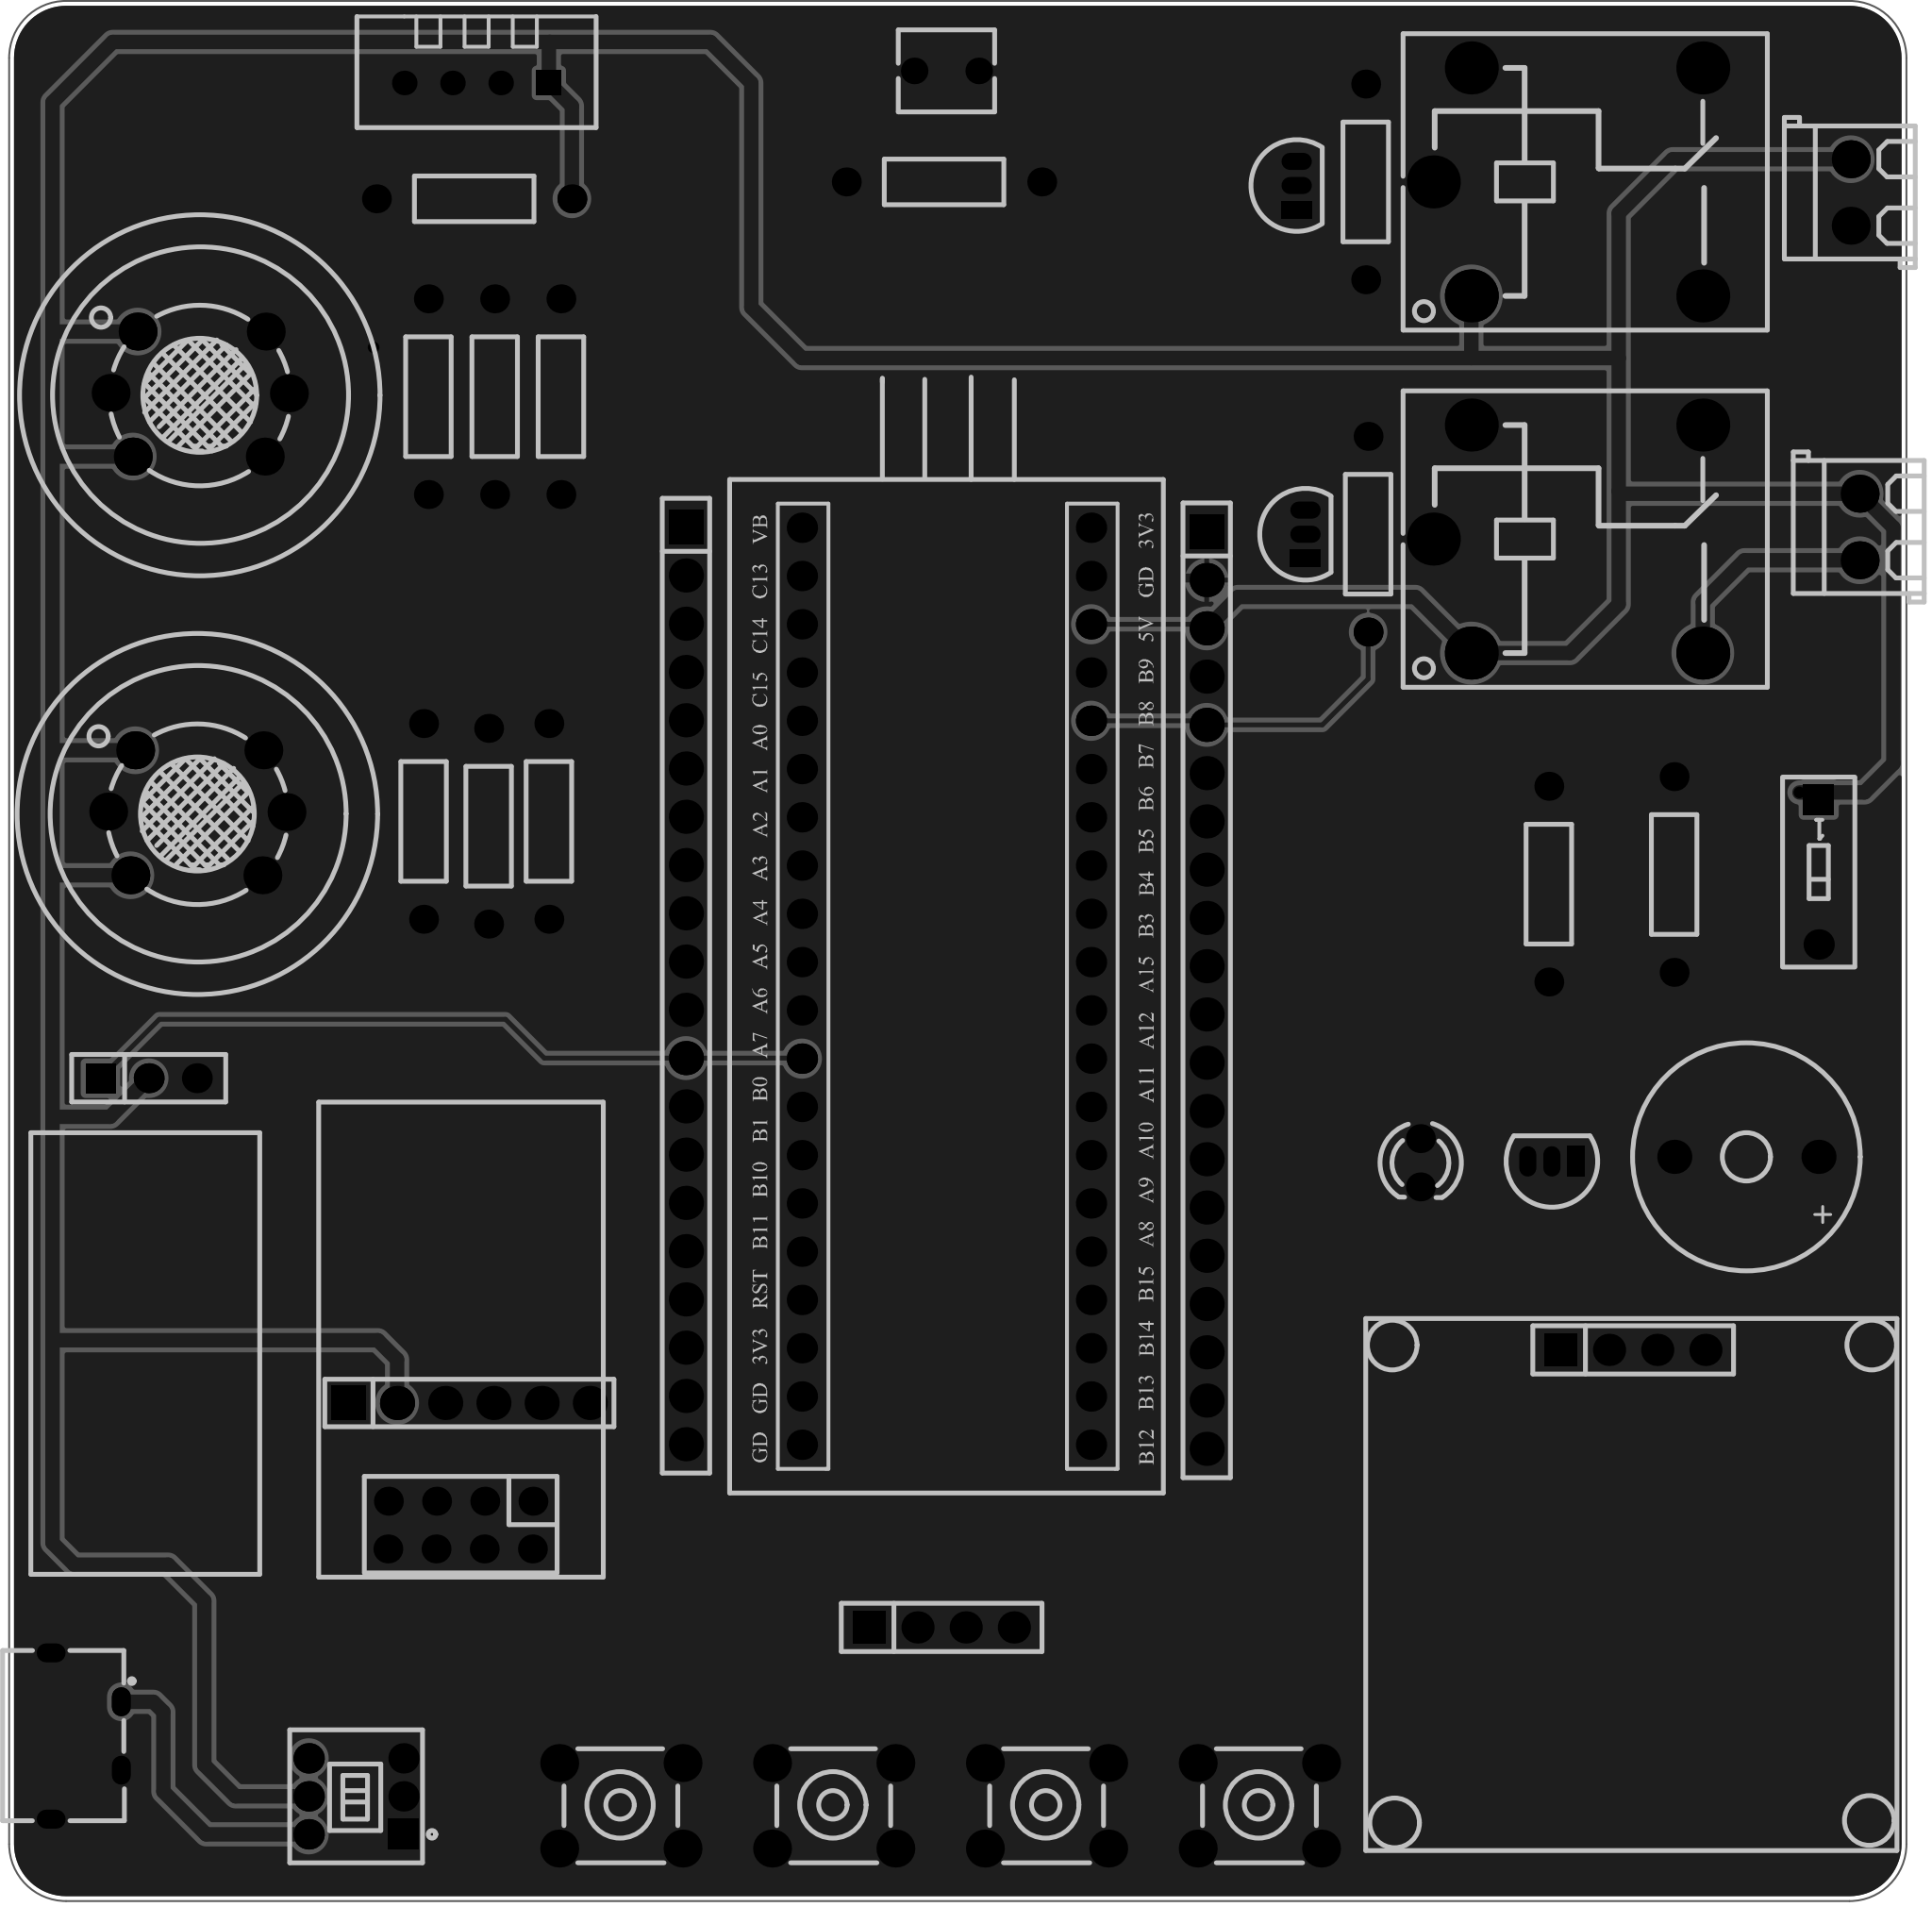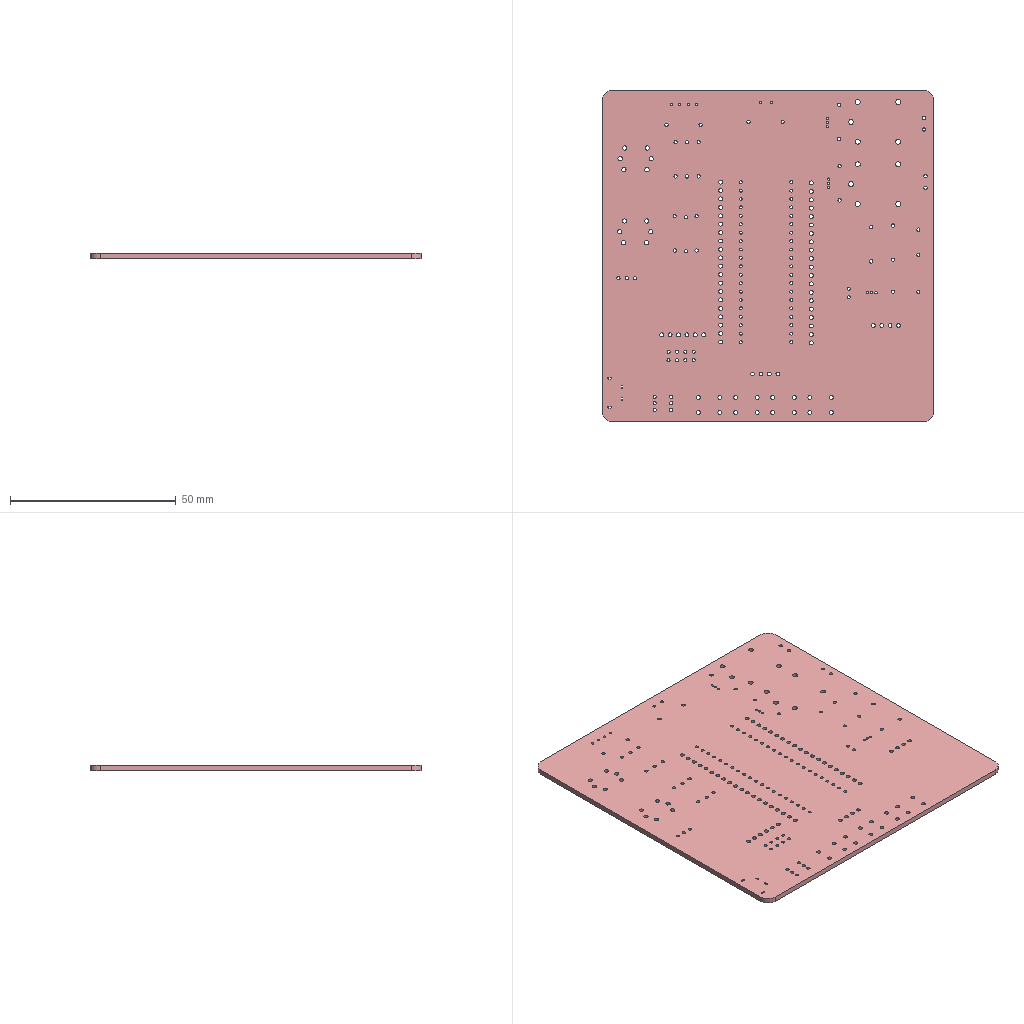Circuit board layout | Altium Designer | box 100 x 100 x 1.6 mm
Layer stack:
# Altium Designer layer stack of  (unit mm; dielectric type: 0 none, 1 core, 2 prepreg, 3 surface material)
index,name,kind,layer,copper_thickness_mm,dielectric_type,dielectric_thickness_mm,dielectric_material,dielectric_constant
0,Top Paste Mask Layer,other,,,,,,
1,Top Silkscreen Layer,other,,,,,,
2,Top Solder Mask Layer,dielectric,,,3,0.01,,3.3
3,Top Layer,copper,Top Layer,0.035,,,,
4,Dielectric1,dielectric,,,3,1.51,FR4,4.5
5,Bottom Layer,copper,Bottom Layer,0.035,,,,
6,Bottom Solder Mask Layer,dielectric,,,3,0.01,,3.3
7,Bottom Silkscreen Layer,other,,,,,,
8,Bottom Paste Mask Layer,other,,,,,,
# drill layer pairs: low layer,high layer
drill_pair,Top Layer,Bottom Layer
Part placement:
Designator,Comment,Layer,Footprint,Center-X(mm),Center-Y(mm),Rotation
USB1,KH-TYPE-C-2P,TopLayer,USB-SMD_KH-TYPE-C-2P,87.757,93.345,270
H6,,TopLayer,HDR-TH_3P-P2.54-V-F,91.048,127.962,0
U1,MQ-2,TopLayer,SENSOR-TH_MQ-2,93.614,141.932,0
U2,MQ-5,TopLayer,SENSOR-TH_MQ-2,93.741,163.967,0
SW8,TK-6700-1,TopLayer,SW-TH_TK-6700-1,101.981,90.17,90
H13,,TopLayer,HDR-TH_6P-P2.54-V-M-1,107.95,110.871,0
R13,10kΩ,TopLayer,Res_1/4W,108.204,174.244,0
U98,,TopLayer,WiFi封装,107.479,104.445,0
U7,DHT11,TopLayer,SENSOR-TH_DHT11,108.331,180.34,180
R3,5Ω,TopLayer,Res_1/4W,105.537,141.478,90
R6,5Ω,TopLayer,Res_1/4W,105.791,163.83,90
R1,10kΩ,TopLayer,Res_1/4W,108.966,141.224,90
R4,10kΩ,TopLayer,Res_1/4W,109.284,163.83,90
R2,10kΩ,TopLayer,Res_1/4W,112.141,141.478,90
KEY1,Button 1,TopLayer,KEY-TH_4P-L6.0-W6.0-P4.50-LS7.5,115.937,89.672,0
R5,10kΩ,TopLayer,Res_1/4W,112.776,163.83,90
H4,,TopLayer,HDR-TH_20P-P2.54-V-F,119.366,132.831,270
KEY5,Button 5,TopLayer,KEY-TH_4P-L6.0-W6.0-P4.50-LS7.5,127.156,89.672,0
U44,,TopLayer,STM32最小系统板,133.098,132.803,0
R7,1kΩ,TopLayer,Res_1/4W,132.969,175.133,180
H7,,TopLayer,HDR-TH_4P-P2.54-V-F,132.842,99.06,0
U3,光敏电阻-5MM,TopLayer,RES-TH_L4.9-W4.3-P3.4,133.096,180.975,180
KEY3,Button 2,TopLayer,KEY-TH_4P-L6.0-W6.0-P4.50-LS7.5,138.374,89.672,0
KEY4,Button 4,TopLayer,KEY-TH_4P-L6.0-W6.0-P4.50-LS7.5,149.592,89.672,0
H3,,TopLayer,HDR-TH_20P-P2.54-V-F,146.812,132.588,270
Q2,,TopLayer,S8050_TO_92,151.556,174.944,90
Q3,,TopLayer,S8050_TO_92,152.019,156.591,90
R15,1kΩ,TopLayer,Res_1/4W,155.194,175.133,90
R10,1kΩ,TopLayer,Res_1/4W,155.321,156.591,90
LED1,,TopLayer,LED_TH-3mm,158.077,123.513,270
RLY2,SRD-05VDC-SL-C,TopLayer,RELAY-TH_SRD-XXVDC-XL-C,165.862,156.337,0
RLY1,SRD-05VDC-SL-C,TopLayer,RELAY-TH_SRD-XXVDC-XL-C,165.862,175.133,0
Q1,,TopLayer,S8050_TO_92,165.006,123.586,180
R9,120,TopLayer,Res_1/4W,164.846,138.176,270
H10,2.54-1*4P female,TopLayer,HDR-TH_4P-P2.54-V-F,169.291,113.665,0
R8,1kΩ,TopLayer,Res_1/4W,171.45,138.684,270
BUZZER1,2.3kHz,TopLayer,BUZ-TH_BD12.0-P7.60-D0.6-FD,175.26,123.825,180
SW5,NDS-01V,TopLayer,SW-TH_2P-L3.9-W9.9-P2.54-LS7.6,179.07,138.811,270
U4,KF350-3.5-2P,TopLayer,CONN-TH_P3.50_KF350-3.5-2P,180.759,174.577,90
U5,KF350-3.5-2P,TopLayer,CONN-TH_P3.50_KF350-3.5-2P,181.229,156.972,90
Pad and via stacks:
# Altium Designer via and pad stacks of  (unit mm). Each distinct definition once, with the count of objects using it.
# via: kind,start_layer,end_layer,hole_mm,diameter_mm,mode(0 simple;1 top-mid-bottom;2 full stack),diameter_per_layer,count,example_net
# pad: kind,layer,hole_mm,hole_type(0 round;1 square;2 slot),plating,top_size,top_shape(1 round;2 rect;3 octagon;9 rounded rect),mid_size,bottom_size,mode,footprint,size_per_layer,count,example
pad,Multi-Layer,0.45,2,plated,1x1.524,1,1x1.524,1x1.524,0,USB-SMD_KH-TYPE-C-2P,,2,USB1.1
pad,Multi-Layer,0.5,2,plated,1x1.524,1,1x1.524,1x1.524,0,USB-SMD_KH-TYPE-C-2P,,2,USB1.3
pad,Multi-Layer,1.02,0,plated,1.575x1.575,1,1.575x1.575,1.575x1.575,0,HDR-TH_3P-P2.54-V-F,,2,H6.3
pad,Multi-Layer,1.02,0,plated,1.575x1.575,2,1.575x1.575,1.575x1.575,0,HDR-TH_3P-P2.54-V-F,,1,H6.1
pad,Multi-Layer,1.3,0,plated,2x2,1,2x2,2x2,0,SENSOR-TH_MQ-2,,12,U1.1
pad,Multi-Layer,1,0,plated,1.6x1.6,2,1.6x1.6,1.6x1.6,0,SW-TH_TK-6700-1,,1,SW8.1
pad,Multi-Layer,1,0,plated,1.6x1.6,1,1.6x1.6,1.6x1.6,0,SW-TH_TK-6700-1,,5,SW8.2
pad,Multi-Layer,1.2,0,plated,1.8x1.8,1,1.8x1.8,1.8x1.8,0,HDR-TH_6P-P2.54-V-M-1,,5,H13.6
pad,Multi-Layer,1.2,0,plated,1.8x1.8,2,1.8x1.8,1.8x1.8,0,HDR-TH_6P-P2.54-V-M-1,,1,H13.1
pad,Multi-Layer,1,0,plated,1.524x1.524,1,1.524x1.524,1.524x1.524,0,Res_1/4W,,24,R13.1
pad,Multi-Layer,0.9144,0,plated,1.524x1.524,1,1.524x1.524,1.524x1.524,0,WiFi\u00B7\u00E2\u00D7\u00B0,,8,U98.1
pad,Multi-Layer,0.7112,0,plated,1.295x1.295,2,1.295x1.295,1.295x1.295,0,SENSOR-TH_DHT11,,1,U7.1
pad,Multi-Layer,0.7112,0,plated,1.295x1.295,1,1.295x1.295,1.295x1.295,0,SENSOR-TH_DHT11,,3,U7.2
pad,Multi-Layer,1.2,0,plated,2x2,1,2x2,2x2,0,KEY-TH_4P-L6.0-W6.0-P4.50-LS7.5,,16,KEY1.1
pad,Multi-Layer,1.2,0,plated,1.8x1.8,2,1.8x1.8,1.8x1.8,0,HDR-TH_20P-P2.54-V-F,,2,H4.1
pad,Multi-Layer,1.2,0,plated,1.8x1.8,1,1.8x1.8,1.8x1.8,0,HDR-TH_20P-P2.54-V-F,,38,H4.2
pad,Multi-Layer,0.9,0,plated,1.6x1.6,1,1.6x1.6,1.6x1.6,0,STM32\u00D7\u00EE\u00D0\u00A1\u00CF\u00B5\u00CD\u00B3\u00B0\u00E5,,40,U44.40
pad,Multi-Layer,1.1,0,plated,1.7x1.7,2,1.7x1.7,1.7x1.7,0,HDR-TH_4P-P2.54-V-F,,2,H7.1
pad,Multi-Layer,1.1,0,plated,1.7x1.7,1,1.7x1.7,1.7x1.7,0,HDR-TH_4P-P2.54-V-F,,6,H7.2
pad,Multi-Layer,0.8,0,plated,1.4x1.4,1,1.4x1.4,1.4x1.4,0,RES-TH_L4.9-W4.3-P3.4,,2,U3.1
pad,Multi-Layer,0.701,0,plated,0.8992x1.6,2,0.8992x1.6,0.8992x1.6,0,S8050_TO_92,,3,Q2.1
pad,Multi-Layer,0.701,0,plated,0.8992x1.6,1,0.8992x1.6,0.8992x1.6,0,S8050_TO_92,,6,Q2.2
pad,Multi-Layer,0.9144,0,plated,1.524x1.524,1,1.524x1.524,1.524x1.524,0,LED_TH-3mm,,2,LED1.1
pad,Multi-Layer,1.524,0,plated,2.794x2.794,1,2.794x2.794,2.794x2.794,0,RELAY-TH_SRD-XXVDC-XL-C,,10,RLY2.2
pad,Multi-Layer,1,0,plated,1.8x1.8,1,1.8x1.8,1.8x1.8,0,BUZ-TH_BD12.0-P7.60-D0.6-FD,,2,BUZZER1.2
pad,Multi-Layer,1,0,plated,1.6x1.6,2,1.6x1.6,1.6x1.6,0,SW-TH_2P-L3.9-W9.9-P2.54-LS7.6,,1,SW5.1
pad,Multi-Layer,1,0,plated,1.6x1.6,1,1.6x1.6,1.6x1.6,0,SW-TH_2P-L3.9-W9.9-P2.54-LS7.6,,1,SW5.2
pad,Multi-Layer,1,0,plated,2x2,1,2x2,2x2,0,CONN-TH_P3.50_KF350-3.5-2P,,4,U4.1
via,Top Layer,Bottom Layer,0.3048,0.61,0,,2,GND
Copper pours:
name,layer,net,type(0 solid;1 hatched;2 none)
Bottom Layer-GND,Bottom Layer,GND,0
Top Layer-GND,Top Layer,GND,0
Design rules, without the lines most boards share:
# Altium Designer design rules of  (exported by Altium Designer, unit mm)
# columns: name | kind | enabled | priority | scope1 | scope2 | descriptor | typed fields (field=value)
creepage | 65 | enabled | 1 | All | All | Creepage Distance Constraint =(0mil) (All),(All) |